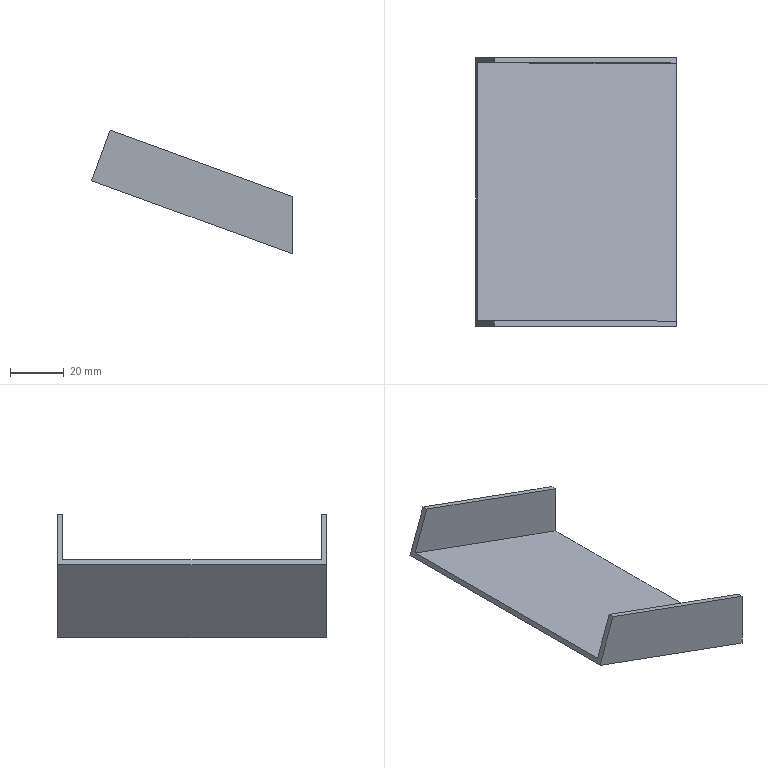Part | NX | features solid 2 | 1 solid | 10 faces | box 74.698 x 100 x 45.982 mm | volume 21261 mm3 | plane 10
STEP:
#1=CARTESIAN_POINT('',(602.142,-110.,-159.496));
#2=VERTEX_POINT('',#1);
#3=CARTESIAN_POINT('',(595.302,-110.,-178.29));
#4=VERTEX_POINT('',#3);
#5=CARTESIAN_POINT('',(595.986,-110.,-176.411));
#6=DIRECTION('',(-0.342,0.,-0.9397));
#7=VECTOR('',#6,1000.);
#8=LINE('',#5,#7);
#9=EDGE_CURVE('',#2,#4,#8,.T.);
#10=ORIENTED_EDGE('',*,*,#9,.T.);
#11=CARTESIAN_POINT('',(670.,-110.,-205.478));
#12=VERTEX_POINT('',#11);
#13=CARTESIAN_POINT('',(1413.3,-110.,-476.017));
#14=DIRECTION('',(-0.9397,0.,0.342));
#15=VECTOR('',#14,1000.);
#16=LINE('',#13,#15);
#17=EDGE_CURVE('',#12,#4,#16,.T.);
#18=ORIENTED_EDGE('',*,*,#17,.F.);
#19=CARTESIAN_POINT('',(670.,-110.,-184.194));
#20=VERTEX_POINT('',#19);
#21=CARTESIAN_POINT('',(670.,-110.,-216.397));
#22=DIRECTION('',(0.,0.,1.));
#23=VECTOR('',#22,1000.);
#24=LINE('',#21,#23);
#25=EDGE_CURVE('',#12,#20,#24,.T.);
#26=ORIENTED_EDGE('',*,*,#25,.T.);
#27=CARTESIAN_POINT('',(2183.44,-110.,-735.042));
#28=DIRECTION('',(-0.9397,0.,0.342));
#29=VECTOR('',#28,1000.);
#30=LINE('',#27,#29);
#31=EDGE_CURVE('',#20,#2,#30,.T.);
#32=ORIENTED_EDGE('',*,*,#31,.T.);
#33=EDGE_LOOP('',(#10,#18,#26,#32));
#34=FACE_BOUND('',#33,.T.);
#35=CARTESIAN_POINT('',(2177.284,-110.,-751.956));
#36=DIRECTION('',(0.,1.,0.));
#37=DIRECTION('',(0.,0.,1.));
#38=AXIS2_PLACEMENT_3D('',#35,#36,#37);
#39=PLANE('',#38);
#40=ADVANCED_FACE('',(#34),#39,.F.);
#41=CARTESIAN_POINT('',(670.,-10.,-205.478));
#42=VERTEX_POINT('',#41);
#43=CARTESIAN_POINT('',(670.,-10.,-184.194));
#44=VERTEX_POINT('',#43);
#45=CARTESIAN_POINT('',(670.,-10.,-216.397));
#46=DIRECTION('',(0.,0.,1.));
#47=VECTOR('',#46,1000.);
#48=LINE('',#45,#47);
#49=EDGE_CURVE('',#42,#44,#48,.T.);
#50=ORIENTED_EDGE('',*,*,#49,.F.);
#51=CARTESIAN_POINT('',(595.302,-10.,-178.29));
#52=VERTEX_POINT('',#51);
#53=CARTESIAN_POINT('',(1413.3,-10.,-476.017));
#54=DIRECTION('',(-0.9397,0.,0.342));
#55=VECTOR('',#54,1000.);
#56=LINE('',#53,#55);
#57=EDGE_CURVE('',#42,#52,#56,.T.);
#58=ORIENTED_EDGE('',*,*,#57,.T.);
#59=CARTESIAN_POINT('',(602.142,-10.,-159.496));
#60=VERTEX_POINT('',#59);
#61=CARTESIAN_POINT('',(595.986,-10.,-176.411));
#62=DIRECTION('',(-0.342,0.,-0.9397));
#63=VECTOR('',#62,1000.);
#64=LINE('',#61,#63);
#65=EDGE_CURVE('',#60,#52,#64,.T.);
#66=ORIENTED_EDGE('',*,*,#65,.F.);
#67=CARTESIAN_POINT('',(706.84,-10.,-197.603));
#68=DIRECTION('',(-0.9397,0.,0.342));
#69=VECTOR('',#68,1000.);
#70=LINE('',#67,#69);
#71=EDGE_CURVE('',#44,#60,#70,.T.);
#72=ORIENTED_EDGE('',*,*,#71,.F.);
#73=EDGE_LOOP('',(#50,#58,#66,#72));
#74=FACE_BOUND('',#73,.T.);
#75=CARTESIAN_POINT('',(2177.284,-10.,-751.956));
#76=DIRECTION('',(0.,1.,0.));
#77=DIRECTION('',(0.,0.,1.));
#78=AXIS2_PLACEMENT_3D('',#75,#76,#77);
#79=PLANE('',#78);
#80=ADVANCED_FACE('',(#74),#79,.T.);
#81=CARTESIAN_POINT('',(602.142,-108.,-159.496));
#82=VERTEX_POINT('',#81);
#83=CARTESIAN_POINT('',(595.986,-108.,-176.411));
#84=VERTEX_POINT('',#83);
#85=CARTESIAN_POINT('',(595.302,-108.,-178.29));
#86=DIRECTION('',(-0.342,0.,-0.9397));
#87=VECTOR('',#86,1000.);
#88=LINE('',#85,#87);
#89=EDGE_CURVE('',#82,#84,#88,.T.);
#90=ORIENTED_EDGE('',*,*,#89,.T.);
#91=CARTESIAN_POINT('',(595.986,-12.,-176.411));
#92=VERTEX_POINT('',#91);
#93=CARTESIAN_POINT('',(595.986,-606.946,-176.411));
#94=DIRECTION('',(0.,1.,0.));
#95=VECTOR('',#94,1000.);
#96=LINE('',#93,#95);
#97=EDGE_CURVE('',#84,#92,#96,.T.);
#98=ORIENTED_EDGE('',*,*,#97,.T.);
#99=CARTESIAN_POINT('',(602.142,-12.,-159.496));
#100=VERTEX_POINT('',#99);
#101=CARTESIAN_POINT('',(595.986,-12.,-176.411));
#102=DIRECTION('',(-0.342,0.,-0.9397));
#103=VECTOR('',#102,1000.);
#104=LINE('',#101,#103);
#105=EDGE_CURVE('',#100,#92,#104,.T.);
#106=ORIENTED_EDGE('',*,*,#105,.F.);
#107=CARTESIAN_POINT('',(602.142,10.,-159.496));
#108=DIRECTION('',(0.,1.,0.));
#109=VECTOR('',#108,1000.);
#110=LINE('',#107,#109);
#111=EDGE_CURVE('',#100,#60,#110,.T.);
#112=ORIENTED_EDGE('',*,*,#111,.T.);
#113=ORIENTED_EDGE('',*,*,#65,.T.);
#114=CARTESIAN_POINT('',(595.302,-606.946,-178.29));
#115=DIRECTION('',(0.,1.,0.));
#116=VECTOR('',#115,1000.);
#117=LINE('',#114,#116);
#118=EDGE_CURVE('',#4,#52,#117,.T.);
#119=ORIENTED_EDGE('',*,*,#118,.F.);
#120=ORIENTED_EDGE('',*,*,#9,.F.);
#121=CARTESIAN_POINT('',(602.142,-90.,-159.496));
#122=DIRECTION('',(0.,-1.,0.));
#123=VECTOR('',#122,1000.);
#124=LINE('',#121,#123);
#125=EDGE_CURVE('',#82,#2,#124,.T.);
#126=ORIENTED_EDGE('',*,*,#125,.F.);
#127=EDGE_LOOP('',(#90,#98,#106,#112,#113,#119,#120,#126));
#128=FACE_BOUND('',#127,.T.);
#129=CARTESIAN_POINT('',(595.986,-2257.783,-176.411));
#130=DIRECTION('',(0.9397,0.,-0.342));
#131=DIRECTION('',(0.342,0.,0.9397));
#132=AXIS2_PLACEMENT_3D('',#129,#130,#131);
#133=PLANE('',#132);
#134=ADVANCED_FACE('',(#128),#133,.F.);
#135=ORIENTED_EDGE('',*,*,#105,.T.);
#136=CARTESIAN_POINT('',(670.,-12.,-203.35));
#137=VERTEX_POINT('',#136);
#138=CARTESIAN_POINT('',(1413.984,-12.,-474.138));
#139=DIRECTION('',(-0.9397,0.,0.342));
#140=VECTOR('',#139,1000.);
#141=LINE('',#138,#140);
#142=EDGE_CURVE('',#137,#92,#141,.T.);
#143=ORIENTED_EDGE('',*,*,#142,.F.);
#144=CARTESIAN_POINT('',(670.,-12.,-184.194));
#145=VERTEX_POINT('',#144);
#146=CARTESIAN_POINT('',(670.,-12.,-216.397));
#147=DIRECTION('',(0.,0.,-1.));
#148=VECTOR('',#147,1000.);
#149=LINE('',#146,#148);
#150=EDGE_CURVE('',#145,#137,#149,.T.);
#151=ORIENTED_EDGE('',*,*,#150,.F.);
#152=CARTESIAN_POINT('',(706.84,-12.,-197.603));
#153=DIRECTION('',(-0.9397,0.,0.342));
#154=VECTOR('',#153,1000.);
#155=LINE('',#152,#154);
#156=EDGE_CURVE('',#145,#100,#155,.T.);
#157=ORIENTED_EDGE('',*,*,#156,.T.);
#158=EDGE_LOOP('',(#135,#143,#151,#157));
#159=FACE_BOUND('',#158,.T.);
#160=CARTESIAN_POINT('',(700.,-12.,-216.397));
#161=DIRECTION('',(0.,1.,0.));
#162=DIRECTION('',(-0.9397,0.,0.342));
#163=AXIS2_PLACEMENT_3D('',#160,#161,#162);
#164=PLANE('',#163);
#165=ADVANCED_FACE('',(#159),#164,.F.);
#166=ORIENTED_EDGE('',*,*,#156,.F.);
#167=CARTESIAN_POINT('',(670.,10.,-184.194));
#168=DIRECTION('',(0.,-1.,0.));
#169=VECTOR('',#168,1000.);
#170=LINE('',#167,#169);
#171=EDGE_CURVE('',#44,#145,#170,.T.);
#172=ORIENTED_EDGE('',*,*,#171,.F.);
#173=ORIENTED_EDGE('',*,*,#71,.T.);
#174=ORIENTED_EDGE('',*,*,#111,.F.);
#175=EDGE_LOOP('',(#166,#172,#173,#174));
#176=FACE_BOUND('',#175,.T.);
#177=CARTESIAN_POINT('',(706.84,10.,-197.603));
#178=DIRECTION('',(-0.342,0.,-0.9397));
#179=DIRECTION('',(0.9397,0.,-0.342));
#180=AXIS2_PLACEMENT_3D('',#177,#178,#179);
#181=PLANE('',#180);
#182=ADVANCED_FACE('',(#176),#181,.F.);
#183=CARTESIAN_POINT('',(670.,-108.,-203.35));
#184=VERTEX_POINT('',#183);
#185=CARTESIAN_POINT('',(1413.984,-108.,-474.138));
#186=DIRECTION('',(0.9397,0.,-0.342));
#187=VECTOR('',#186,1000.);
#188=LINE('',#185,#187);
#189=EDGE_CURVE('',#84,#184,#188,.T.);
#190=ORIENTED_EDGE('',*,*,#189,.F.);
#191=ORIENTED_EDGE('',*,*,#89,.F.);
#192=CARTESIAN_POINT('',(670.,-108.,-184.194));
#193=VERTEX_POINT('',#192);
#194=CARTESIAN_POINT('',(706.84,-108.,-197.603));
#195=DIRECTION('',(-0.9397,0.,0.342));
#196=VECTOR('',#195,1000.);
#197=LINE('',#194,#196);
#198=EDGE_CURVE('',#193,#82,#197,.T.);
#199=ORIENTED_EDGE('',*,*,#198,.F.);
#200=CARTESIAN_POINT('',(670.,-108.,-216.397));
#201=DIRECTION('',(0.,0.,1.));
#202=VECTOR('',#201,1000.);
#203=LINE('',#200,#202);
#204=EDGE_CURVE('',#184,#193,#203,.T.);
#205=ORIENTED_EDGE('',*,*,#204,.F.);
#206=EDGE_LOOP('',(#190,#191,#199,#205));
#207=FACE_BOUND('',#206,.T.);
#208=CARTESIAN_POINT('',(700.,-108.,-216.397));
#209=DIRECTION('',(0.,-1.,0.));
#210=DIRECTION('',(-0.9397,0.,0.342));
#211=AXIS2_PLACEMENT_3D('',#208,#209,#210);
#212=PLANE('',#211);
#213=ADVANCED_FACE('',(#207),#212,.F.);
#214=ORIENTED_EDGE('',*,*,#125,.T.);
#215=ORIENTED_EDGE('',*,*,#31,.F.);
#216=CARTESIAN_POINT('',(670.,-90.,-184.194));
#217=DIRECTION('',(0.,1.,0.));
#218=VECTOR('',#217,1000.);
#219=LINE('',#216,#218);
#220=EDGE_CURVE('',#20,#193,#219,.T.);
#221=ORIENTED_EDGE('',*,*,#220,.T.);
#222=ORIENTED_EDGE('',*,*,#198,.T.);
#223=EDGE_LOOP('',(#214,#215,#221,#222));
#224=FACE_BOUND('',#223,.T.);
#225=CARTESIAN_POINT('',(706.84,-90.,-197.603));
#226=DIRECTION('',(0.342,0.,0.9397));
#227=DIRECTION('',(-0.9397,0.,0.342));
#228=AXIS2_PLACEMENT_3D('',#225,#226,#227);
#229=PLANE('',#228);
#230=ADVANCED_FACE('',(#224),#229,.T.);
#231=ORIENTED_EDGE('',*,*,#142,.T.);
#232=ORIENTED_EDGE('',*,*,#97,.F.);
#233=ORIENTED_EDGE('',*,*,#189,.T.);
#234=CARTESIAN_POINT('',(670.,-606.946,-203.35));
#235=DIRECTION('',(0.,-1.,0.));
#236=VECTOR('',#235,1000.);
#237=LINE('',#234,#236);
#238=EDGE_CURVE('',#137,#184,#237,.T.);
#239=ORIENTED_EDGE('',*,*,#238,.F.);
#240=EDGE_LOOP('',(#231,#232,#233,#239));
#241=FACE_BOUND('',#240,.T.);
#242=CARTESIAN_POINT('',(1413.984,-606.946,-474.138));
#243=DIRECTION('',(-0.342,0.,-0.9397));
#244=DIRECTION('',(0.9397,0.,-0.342));
#245=AXIS2_PLACEMENT_3D('',#242,#243,#244);
#246=PLANE('',#245);
#247=ADVANCED_FACE('',(#241),#246,.F.);
#248=CARTESIAN_POINT('',(670.,-90.,-205.478));
#249=DIRECTION('',(0.,1.,0.));
#250=VECTOR('',#249,1000.);
#251=LINE('',#248,#250);
#252=EDGE_CURVE('',#12,#42,#251,.T.);
#253=ORIENTED_EDGE('',*,*,#252,.F.);
#254=ORIENTED_EDGE('',*,*,#17,.T.);
#255=ORIENTED_EDGE('',*,*,#118,.T.);
#256=ORIENTED_EDGE('',*,*,#57,.F.);
#257=EDGE_LOOP('',(#253,#254,#255,#256));
#258=FACE_BOUND('',#257,.T.);
#259=CARTESIAN_POINT('',(1413.3,-606.946,-476.017));
#260=DIRECTION('',(-0.342,0.,-0.9397));
#261=DIRECTION('',(0.9397,0.,-0.342));
#262=AXIS2_PLACEMENT_3D('',#259,#260,#261);
#263=PLANE('',#262);
#264=ADVANCED_FACE('',(#258),#263,.T.);
#265=ORIENTED_EDGE('',*,*,#49,.T.);
#266=ORIENTED_EDGE('',*,*,#171,.T.);
#267=ORIENTED_EDGE('',*,*,#150,.T.);
#268=ORIENTED_EDGE('',*,*,#238,.T.);
#269=ORIENTED_EDGE('',*,*,#204,.T.);
#270=ORIENTED_EDGE('',*,*,#220,.F.);
#271=ORIENTED_EDGE('',*,*,#25,.F.);
#272=ORIENTED_EDGE('',*,*,#252,.T.);
#273=EDGE_LOOP('',(#265,#266,#267,#268,#269,#270,#271,#272));
#274=FACE_BOUND('',#273,.T.);
#275=CARTESIAN_POINT('',(670.,-90.,-216.397));
#276=DIRECTION('',(-1.,0.,0.));
#277=DIRECTION('',(0.,0.,-1.));
#278=AXIS2_PLACEMENT_3D('',#275,#276,#277);
#279=PLANE('',#278);
#280=ADVANCED_FACE('',(#274),#279,.F.);
#281=CLOSED_SHELL('',(#40,#80,#134,#165,#182,#213,#230,#247,#264,#280));
#282=MANIFOLD_SOLID_BREP('',#281);
#283=(LENGTH_UNIT()NAMED_UNIT(*)SI_UNIT(.MILLI.,.METRE.));
#284=UNCERTAINTY_MEASURE_WITH_UNIT(LENGTH_MEASURE(0.00001),#283,'','');
#285=(NAMED_UNIT(*)PLANE_ANGLE_UNIT()SI_UNIT($,.RADIAN.));
#286=(NAMED_UNIT(*)SI_UNIT($,.STERADIAN.)SOLID_ANGLE_UNIT());
#287=(GEOMETRIC_REPRESENTATION_CONTEXT(3)GLOBAL_UNCERTAINTY_ASSIGNED_CONTEXT((#284))GLOBAL_UNIT_ASSIGNED_CONTEXT((#283,#285,#286))REPRESENTATION_CONTEXT('',''));
#288=ADVANCED_BREP_SHAPE_REPRESENTATION('',(#282),#287);